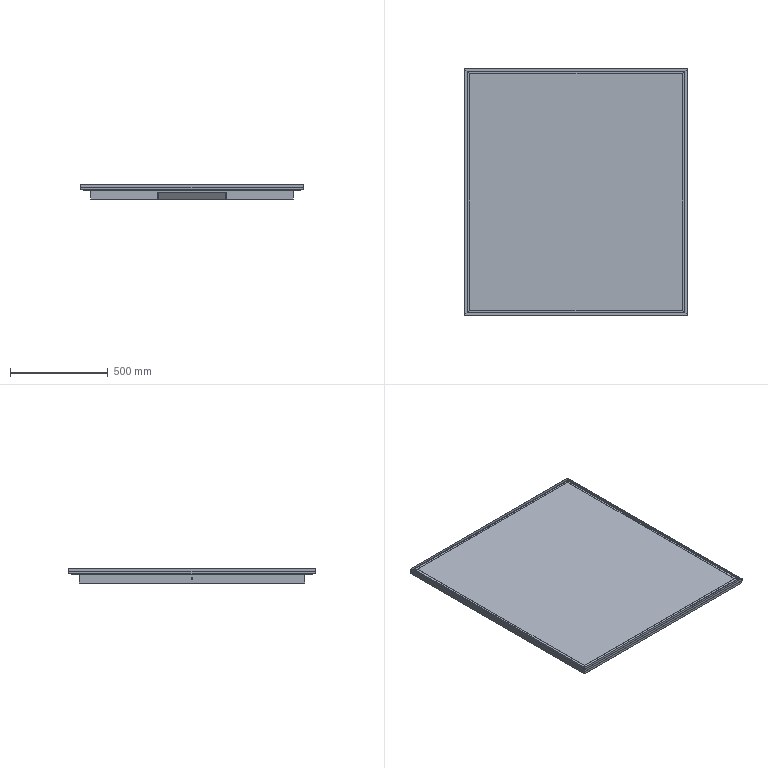Part | SolidWorks | 7 solids | 282 faces | box 1140 x 1260 x 75 mm | volume 31682872 mm3 | plane 148 | cylinder 122 | spline 12 | commonest cylinder face diameters 4.2 x80 11 x14 0.4 x11 2.4 x11 10 x6